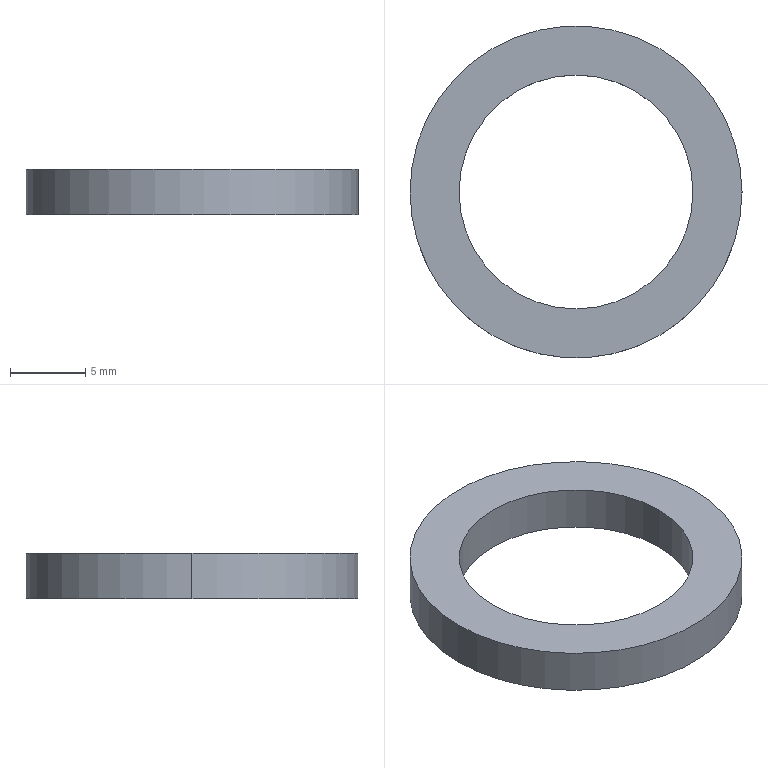Part | SolidWorks | features Extrusion 1 | 1 solid | 6 faces | box 22 x 22 x 3 mm | volume 574.322 mm3 | cylinder 4 | plane 2 | commonest cylinder face diameters 15.5 x2 22 x2
STEP:
#1=CARTESIAN_POINT('',(-7.75,0.,3.));
#2=VERTEX_POINT('',#1);
#3=CARTESIAN_POINT('',(7.75,0.,3.));
#4=VERTEX_POINT('',#3);
#5=CARTESIAN_POINT('',(0.,0.,3.));
#6=DIRECTION('',(0.,0.,1.));
#7=DIRECTION('',(1.,0.,0.));
#8=AXIS2_PLACEMENT_3D('',#5,#6,#7);
#9=CIRCLE('',#8,7.75);
#10=EDGE_CURVE('',#2,#4,#9,.T.);
#11=ORIENTED_EDGE('',*,*,#10,.T.);
#12=CARTESIAN_POINT('',(7.75,0.,0.));
#13=VERTEX_POINT('',#12);
#14=CARTESIAN_POINT('',(7.75,0.,3.));
#15=DIRECTION('',(0.,0.,-1.));
#16=VECTOR('',#15,1000.);
#17=LINE('',#14,#16);
#18=EDGE_CURVE('',#4,#13,#17,.T.);
#19=ORIENTED_EDGE('',*,*,#18,.T.);
#20=CARTESIAN_POINT('',(-7.75,0.,0.));
#21=VERTEX_POINT('',#20);
#22=CARTESIAN_POINT('',(0.,0.,0.));
#23=DIRECTION('',(0.,0.,1.));
#24=DIRECTION('',(1.,0.,0.));
#25=AXIS2_PLACEMENT_3D('',#22,#23,#24);
#26=CIRCLE('',#25,7.75);
#27=EDGE_CURVE('',#21,#13,#26,.T.);
#28=ORIENTED_EDGE('',*,*,#27,.F.);
#29=CARTESIAN_POINT('',(-7.75,0.,3.));
#30=DIRECTION('',(0.,0.,-1.));
#31=VECTOR('',#30,1000.);
#32=LINE('',#29,#31);
#33=EDGE_CURVE('',#2,#21,#32,.T.);
#34=ORIENTED_EDGE('',*,*,#33,.F.);
#35=EDGE_LOOP('',(#11,#19,#28,#34));
#36=FACE_OUTER_BOUND('',#35,.T.);
#37=CARTESIAN_POINT('',(0.,0.,3.));
#38=DIRECTION('',(0.,0.,-1.));
#39=DIRECTION('',(-1.,0.,0.));
#40=AXIS2_PLACEMENT_3D('',#37,#38,#39);
#41=CYLINDRICAL_SURFACE('',#40,7.75);
#42=ADVANCED_FACE('',(#36),#41,.F.);
#43=CARTESIAN_POINT('',(11.,0.,3.));
#44=VERTEX_POINT('',#43);
#45=CARTESIAN_POINT('',(-11.,0.,3.));
#46=VERTEX_POINT('',#45);
#47=CARTESIAN_POINT('',(0.,0.,3.));
#48=DIRECTION('',(0.,0.,1.));
#49=DIRECTION('',(1.,0.,0.));
#50=AXIS2_PLACEMENT_3D('',#47,#48,#49);
#51=CIRCLE('',#50,11.);
#52=EDGE_CURVE('',#44,#46,#51,.T.);
#53=ORIENTED_EDGE('',*,*,#52,.F.);
#54=CARTESIAN_POINT('',(11.,0.,0.));
#55=VERTEX_POINT('',#54);
#56=CARTESIAN_POINT('',(11.,0.,3.));
#57=DIRECTION('',(0.,0.,-1.));
#58=VECTOR('',#57,1000.);
#59=LINE('',#56,#58);
#60=EDGE_CURVE('',#44,#55,#59,.T.);
#61=ORIENTED_EDGE('',*,*,#60,.T.);
#62=CARTESIAN_POINT('',(-11.,0.,0.));
#63=VERTEX_POINT('',#62);
#64=CARTESIAN_POINT('',(0.,0.,0.));
#65=DIRECTION('',(0.,0.,1.));
#66=DIRECTION('',(1.,0.,0.));
#67=AXIS2_PLACEMENT_3D('',#64,#65,#66);
#68=CIRCLE('',#67,11.);
#69=EDGE_CURVE('',#55,#63,#68,.T.);
#70=ORIENTED_EDGE('',*,*,#69,.T.);
#71=CARTESIAN_POINT('',(-11.,0.,3.));
#72=DIRECTION('',(0.,0.,-1.));
#73=VECTOR('',#72,1000.);
#74=LINE('',#71,#73);
#75=EDGE_CURVE('',#46,#63,#74,.T.);
#76=ORIENTED_EDGE('',*,*,#75,.F.);
#77=EDGE_LOOP('',(#53,#61,#70,#76));
#78=FACE_OUTER_BOUND('',#77,.T.);
#79=CARTESIAN_POINT('',(0.,0.,3.));
#80=DIRECTION('',(0.,0.,-1.));
#81=DIRECTION('',(-1.,0.,0.));
#82=AXIS2_PLACEMENT_3D('',#79,#80,#81);
#83=CYLINDRICAL_SURFACE('',#82,11.);
#84=ADVANCED_FACE('',(#78),#83,.T.);
#85=CARTESIAN_POINT('',(0.,0.,3.));
#86=DIRECTION('',(0.,0.,1.));
#87=DIRECTION('',(1.,0.,0.));
#88=AXIS2_PLACEMENT_3D('',#85,#86,#87);
#89=CIRCLE('',#88,11.);
#90=EDGE_CURVE('',#46,#44,#89,.T.);
#91=ORIENTED_EDGE('',*,*,#90,.T.);
#92=ORIENTED_EDGE('',*,*,#52,.T.);
#93=EDGE_LOOP('',(#91,#92));
#94=FACE_OUTER_BOUND('',#93,.T.);
#95=ORIENTED_EDGE('',*,*,#10,.F.);
#96=CARTESIAN_POINT('',(0.,0.,3.));
#97=DIRECTION('',(0.,0.,1.));
#98=DIRECTION('',(1.,0.,0.));
#99=AXIS2_PLACEMENT_3D('',#96,#97,#98);
#100=CIRCLE('',#99,7.75);
#101=EDGE_CURVE('',#4,#2,#100,.T.);
#102=ORIENTED_EDGE('',*,*,#101,.F.);
#103=EDGE_LOOP('',(#95,#102));
#104=FACE_BOUND('',#103,.T.);
#105=CARTESIAN_POINT('',(0.,0.,3.));
#106=DIRECTION('',(0.,0.,1.));
#107=DIRECTION('',(1.,0.,0.));
#108=AXIS2_PLACEMENT_3D('',#105,#106,#107);
#109=PLANE('',#108);
#110=ADVANCED_FACE('',(#94,#104),#109,.T.);
#111=CARTESIAN_POINT('',(0.,0.,0.));
#112=DIRECTION('',(0.,0.,1.));
#113=DIRECTION('',(1.,0.,0.));
#114=AXIS2_PLACEMENT_3D('',#111,#112,#113);
#115=CIRCLE('',#114,11.);
#116=EDGE_CURVE('',#63,#55,#115,.T.);
#117=ORIENTED_EDGE('',*,*,#116,.F.);
#118=ORIENTED_EDGE('',*,*,#69,.F.);
#119=EDGE_LOOP('',(#117,#118));
#120=FACE_OUTER_BOUND('',#119,.T.);
#121=ORIENTED_EDGE('',*,*,#27,.T.);
#122=CARTESIAN_POINT('',(0.,0.,0.));
#123=DIRECTION('',(0.,0.,1.));
#124=DIRECTION('',(1.,0.,0.));
#125=AXIS2_PLACEMENT_3D('',#122,#123,#124);
#126=CIRCLE('',#125,7.75);
#127=EDGE_CURVE('',#13,#21,#126,.T.);
#128=ORIENTED_EDGE('',*,*,#127,.T.);
#129=EDGE_LOOP('',(#121,#128));
#130=FACE_BOUND('',#129,.T.);
#131=CARTESIAN_POINT('',(0.,0.,0.));
#132=DIRECTION('',(0.,0.,1.));
#133=DIRECTION('',(1.,0.,0.));
#134=AXIS2_PLACEMENT_3D('',#131,#132,#133);
#135=PLANE('',#134);
#136=ADVANCED_FACE('',(#120,#130),#135,.F.);
#137=ORIENTED_EDGE('',*,*,#60,.F.);
#138=ORIENTED_EDGE('',*,*,#90,.F.);
#139=ORIENTED_EDGE('',*,*,#75,.T.);
#140=ORIENTED_EDGE('',*,*,#116,.T.);
#141=EDGE_LOOP('',(#137,#138,#139,#140));
#142=FACE_OUTER_BOUND('',#141,.T.);
#143=CARTESIAN_POINT('',(0.,0.,3.));
#144=DIRECTION('',(0.,0.,-1.));
#145=DIRECTION('',(-1.,0.,0.));
#146=AXIS2_PLACEMENT_3D('',#143,#144,#145);
#147=CYLINDRICAL_SURFACE('',#146,11.);
#148=ADVANCED_FACE('',(#142),#147,.T.);
#149=ORIENTED_EDGE('',*,*,#18,.F.);
#150=ORIENTED_EDGE('',*,*,#101,.T.);
#151=ORIENTED_EDGE('',*,*,#33,.T.);
#152=ORIENTED_EDGE('',*,*,#127,.F.);
#153=EDGE_LOOP('',(#149,#150,#151,#152));
#154=FACE_OUTER_BOUND('',#153,.T.);
#155=CARTESIAN_POINT('',(0.,0.,3.));
#156=DIRECTION('',(0.,0.,-1.));
#157=DIRECTION('',(-1.,0.,0.));
#158=AXIS2_PLACEMENT_3D('',#155,#156,#157);
#159=CYLINDRICAL_SURFACE('',#158,7.75);
#160=ADVANCED_FACE('',(#154),#159,.F.);
#161=CLOSED_SHELL('',(#42,#84,#110,#136,#148,#160));
#162=MANIFOLD_SOLID_BREP('',#161);
#163=CARTESIAN_POINT('',(0.,0.,0.));
#164=DIRECTION('',(0.,0.,1.));
#165=DIRECTION('',(1.,0.,0.));
#166=AXIS2_PLACEMENT_3D('',#163,#164,#165);
#167=(LENGTH_UNIT()NAMED_UNIT(*)SI_UNIT(.MILLI.,.METRE.));
#168=UNCERTAINTY_MEASURE_WITH_UNIT(LENGTH_MEASURE(0.00001),#167,'','');
#169=(NAMED_UNIT(*)PLANE_ANGLE_UNIT()SI_UNIT($,.RADIAN.));
#170=(NAMED_UNIT(*)SI_UNIT($,.STERADIAN.)SOLID_ANGLE_UNIT());
#171=(GEOMETRIC_REPRESENTATION_CONTEXT(3)GLOBAL_UNCERTAINTY_ASSIGNED_CONTEXT((#168))GLOBAL_UNIT_ASSIGNED_CONTEXT((#167,#169,#170))REPRESENTATION_CONTEXT('',''));
#172=ADVANCED_BREP_SHAPE_REPRESENTATION('',(#162,#166),#171);